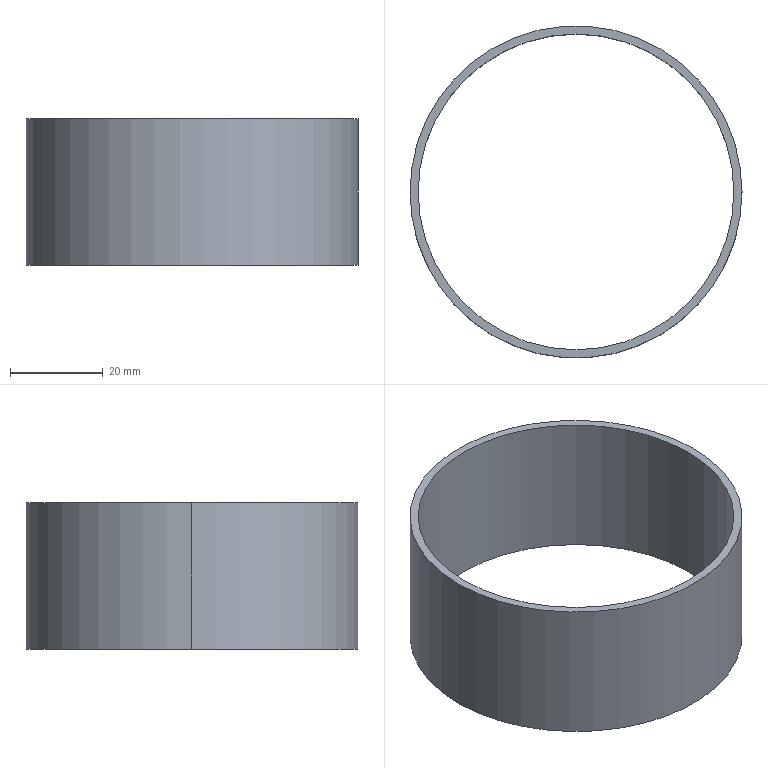Part | STEP file | 20319 | 1 solid | 6 faces | box 71.5 x 71.5 x 31.5 mm | volume 12079 mm3 | cylinder 4 | plane 2 | commonest cylinder face diameters 68 x2 71.5 x2
STEP:
#1=CARTESIAN_POINT('',(35.75,0.,0.));
#2=VERTEX_POINT('',#1);
#3=CARTESIAN_POINT('',(35.75,0.,31.5));
#4=VERTEX_POINT('',#3);
#5=CARTESIAN_POINT('',(35.75,0.,15.75));
#6=DIRECTION('',(0.,0.,1.));
#7=VECTOR('',#6,1.);
#8=LINE('',#5,#7);
#9=EDGE_CURVE('',#2,#4,#8,.T.);
#10=ORIENTED_EDGE('',*,*,#9,.F.);
#11=CARTESIAN_POINT('',(-35.75,0.,0.));
#12=VERTEX_POINT('',#11);
#13=CARTESIAN_POINT('',(0.,0.,0.));
#14=DIRECTION('',(0.,0.,1.));
#15=AXIS2_PLACEMENT_3D('',#13,#14,$);
#16=CIRCLE('',#15,35.75);
#17=EDGE_CURVE('',#2,#12,#16,.T.);
#18=ORIENTED_EDGE('',*,*,#17,.T.);
#19=CARTESIAN_POINT('',(-35.75,0.,31.5));
#20=VERTEX_POINT('',#19);
#21=CARTESIAN_POINT('',(-35.75,0.,15.75));
#22=DIRECTION('',(0.,0.,1.));
#23=VECTOR('',#22,1.);
#24=LINE('',#21,#23);
#25=EDGE_CURVE('',#12,#20,#24,.T.);
#26=ORIENTED_EDGE('',*,*,#25,.T.);
#27=CARTESIAN_POINT('',(0.,0.,31.5));
#28=DIRECTION('',(0.,0.,1.));
#29=AXIS2_PLACEMENT_3D('',#27,#28,$);
#30=CIRCLE('',#29,35.75);
#31=EDGE_CURVE('',#4,#20,#30,.T.);
#32=ORIENTED_EDGE('',*,*,#31,.F.);
#33=EDGE_LOOP('',(#10,#18,#26,#32));
#34=FACE_OUTER_BOUND('',#33,.T.);
#35=CARTESIAN_POINT('',(0.,0.,15.75));
#36=DIRECTION('',(0.,0.,1.));
#37=DIRECTION('',(1.,0.,0.));
#38=AXIS2_PLACEMENT_3D('',#35,#36,#37);
#39=CYLINDRICAL_SURFACE('',#38,35.75);
#40=ADVANCED_FACE('',(#34),#39,.T.);
#41=ORIENTED_EDGE('',*,*,#25,.F.);
#42=CARTESIAN_POINT('',(0.,0.,0.));
#43=DIRECTION('',(0.,0.,1.));
#44=AXIS2_PLACEMENT_3D('',#42,#43,$);
#45=CIRCLE('',#44,35.75);
#46=EDGE_CURVE('',#12,#2,#45,.T.);
#47=ORIENTED_EDGE('',*,*,#46,.T.);
#48=ORIENTED_EDGE('',*,*,#9,.T.);
#49=CARTESIAN_POINT('',(0.,0.,31.5));
#50=DIRECTION('',(0.,0.,1.));
#51=AXIS2_PLACEMENT_3D('',#49,#50,$);
#52=CIRCLE('',#51,35.75);
#53=EDGE_CURVE('',#20,#4,#52,.T.);
#54=ORIENTED_EDGE('',*,*,#53,.F.);
#55=EDGE_LOOP('',(#41,#47,#48,#54));
#56=FACE_OUTER_BOUND('',#55,.T.);
#57=ADVANCED_FACE('',(#56),#39,.T.);
#58=CARTESIAN_POINT('',(-34.,0.,31.5));
#59=VERTEX_POINT('',#58);
#60=CARTESIAN_POINT('',(34.,0.,31.5));
#61=VERTEX_POINT('',#60);
#62=CARTESIAN_POINT('',(0.,0.,31.5));
#63=DIRECTION('',(0.,0.,1.));
#64=AXIS2_PLACEMENT_3D('',#62,#63,$);
#65=CIRCLE('',#64,34.);
#66=EDGE_CURVE('',#59,#61,#65,.T.);
#67=ORIENTED_EDGE('',*,*,#66,.T.);
#68=CARTESIAN_POINT('',(34.,0.,0.));
#69=VERTEX_POINT('',#68);
#70=CARTESIAN_POINT('',(34.,0.,15.75));
#71=DIRECTION('',(0.,0.,1.));
#72=VECTOR('',#71,1.);
#73=LINE('',#70,#72);
#74=EDGE_CURVE('',#69,#61,#73,.T.);
#75=ORIENTED_EDGE('',*,*,#74,.F.);
#76=CARTESIAN_POINT('',(-34.,0.,0.));
#77=VERTEX_POINT('',#76);
#78=CARTESIAN_POINT('',(0.,0.,0.));
#79=DIRECTION('',(0.,0.,1.));
#80=AXIS2_PLACEMENT_3D('',#78,#79,$);
#81=CIRCLE('',#80,34.);
#82=EDGE_CURVE('',#77,#69,#81,.T.);
#83=ORIENTED_EDGE('',*,*,#82,.F.);
#84=CARTESIAN_POINT('',(-34.,0.,15.75));
#85=DIRECTION('',(0.,0.,1.));
#86=VECTOR('',#85,1.);
#87=LINE('',#84,#86);
#88=EDGE_CURVE('',#77,#59,#87,.T.);
#89=ORIENTED_EDGE('',*,*,#88,.T.);
#90=EDGE_LOOP('',(#67,#75,#83,#89));
#91=FACE_OUTER_BOUND('',#90,.T.);
#92=CARTESIAN_POINT('',(0.,0.,15.75));
#93=DIRECTION('',(0.,0.,1.));
#94=DIRECTION('',(1.,0.,0.));
#95=AXIS2_PLACEMENT_3D('',#92,#93,#94);
#96=CYLINDRICAL_SURFACE('',#95,34.);
#97=ADVANCED_FACE('',(#91),#96,.F.);
#98=CARTESIAN_POINT('',(0.,0.,31.5));
#99=DIRECTION('',(0.,0.,1.));
#100=AXIS2_PLACEMENT_3D('',#98,#99,$);
#101=CIRCLE('',#100,34.);
#102=EDGE_CURVE('',#61,#59,#101,.T.);
#103=ORIENTED_EDGE('',*,*,#102,.T.);
#104=ORIENTED_EDGE('',*,*,#88,.F.);
#105=CARTESIAN_POINT('',(0.,0.,0.));
#106=DIRECTION('',(0.,0.,1.));
#107=AXIS2_PLACEMENT_3D('',#105,#106,$);
#108=CIRCLE('',#107,34.);
#109=EDGE_CURVE('',#69,#77,#108,.T.);
#110=ORIENTED_EDGE('',*,*,#109,.F.);
#111=ORIENTED_EDGE('',*,*,#74,.T.);
#112=EDGE_LOOP('',(#103,#104,#110,#111));
#113=FACE_OUTER_BOUND('',#112,.T.);
#114=ADVANCED_FACE('',(#113),#96,.F.);
#115=ORIENTED_EDGE('',*,*,#46,.F.);
#116=ORIENTED_EDGE('',*,*,#17,.F.);
#117=EDGE_LOOP('',(#115,#116));
#118=FACE_OUTER_BOUND('',#117,.T.);
#119=ORIENTED_EDGE('',*,*,#109,.T.);
#120=ORIENTED_EDGE('',*,*,#82,.T.);
#121=EDGE_LOOP('',(#119,#120));
#122=FACE_BOUND('',#121,.T.);
#123=CARTESIAN_POINT('',(0.,0.,0.));
#124=DIRECTION('',(0.,0.,1.));
#125=DIRECTION('',(1.,0.,0.));
#126=AXIS2_PLACEMENT_3D('',#123,#124,#125);
#127=PLANE('',#126);
#128=ADVANCED_FACE('',(#118,#122),#127,.F.);
#129=ORIENTED_EDGE('',*,*,#31,.T.);
#130=ORIENTED_EDGE('',*,*,#53,.T.);
#131=EDGE_LOOP('',(#129,#130));
#132=FACE_OUTER_BOUND('',#131,.T.);
#133=ORIENTED_EDGE('',*,*,#66,.F.);
#134=ORIENTED_EDGE('',*,*,#102,.F.);
#135=EDGE_LOOP('',(#133,#134));
#136=FACE_BOUND('',#135,.T.);
#137=CARTESIAN_POINT('',(0.,0.,31.5));
#138=DIRECTION('',(0.,0.,1.));
#139=DIRECTION('',(1.,0.,0.));
#140=AXIS2_PLACEMENT_3D('',#137,#138,#139);
#141=PLANE('',#140);
#142=ADVANCED_FACE('',(#132,#136),#141,.T.);
#143=CLOSED_SHELL('',(#40,#57,#97,#114,#128,#142));
#144=MANIFOLD_SOLID_BREP('',#143);
#145=(LENGTH_UNIT()NAMED_UNIT(*)SI_UNIT(.MILLI.,.METRE.));
#146=UNCERTAINTY_MEASURE_WITH_UNIT(LENGTH_MEASURE(0.005),#145,'','');
#147=(NAMED_UNIT(*)PLANE_ANGLE_UNIT()SI_UNIT($,.RADIAN.));
#148=(NAMED_UNIT(*)SI_UNIT($,.STERADIAN.)SOLID_ANGLE_UNIT());
#149=(GEOMETRIC_REPRESENTATION_CONTEXT(3)GLOBAL_UNCERTAINTY_ASSIGNED_CONTEXT((#146))GLOBAL_UNIT_ASSIGNED_CONTEXT((#145,#147,#148))REPRESENTATION_CONTEXT('',''));
#150=ADVANCED_BREP_SHAPE_REPRESENTATION('',(#144),#149);